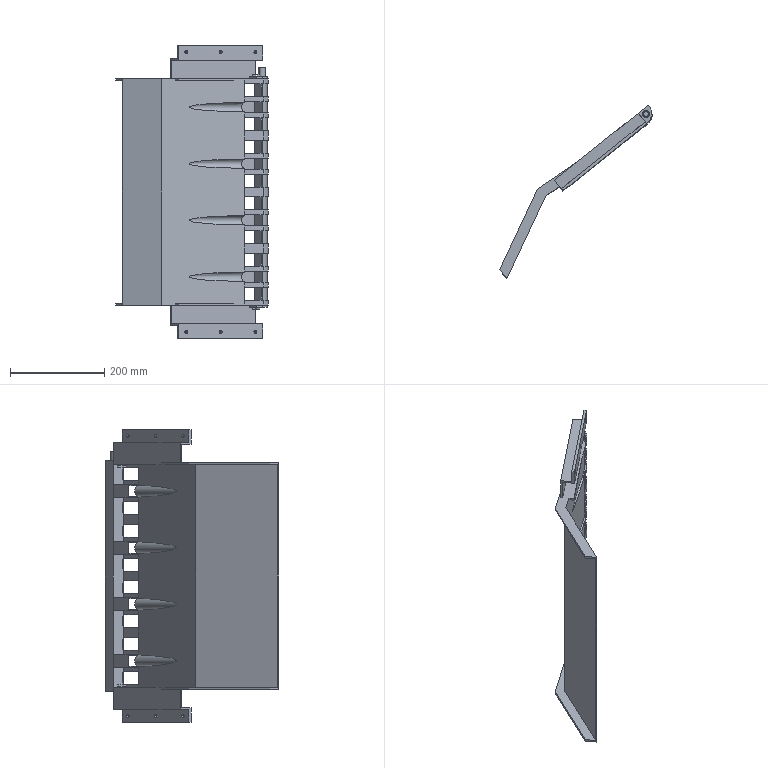Part | SolidWorks | 10 solids | 420 faces | box 323.783 x 368.156 x 620 mm | volume 829181 mm3 | plane 277 | cylinder 133 | cone 10 | commonest cylinder face diameters 5 x40 8 x28 7 x24 55.99 x13 60 x13 20 x4